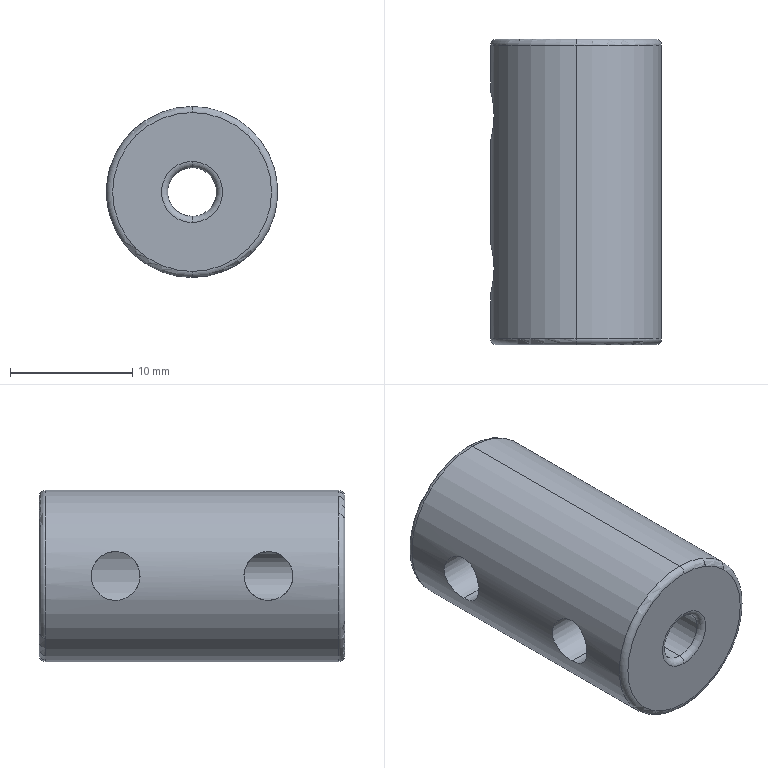Part | STEP file | 48 rigid coupling | 1 solid | 22 faces | box 14 x 25 x 14 mm | volume 2952 mm3 | cylinder 11 | torus 8 | plane 3 | commonest cylinder face diameters 4 x7 8 x2 14 x2